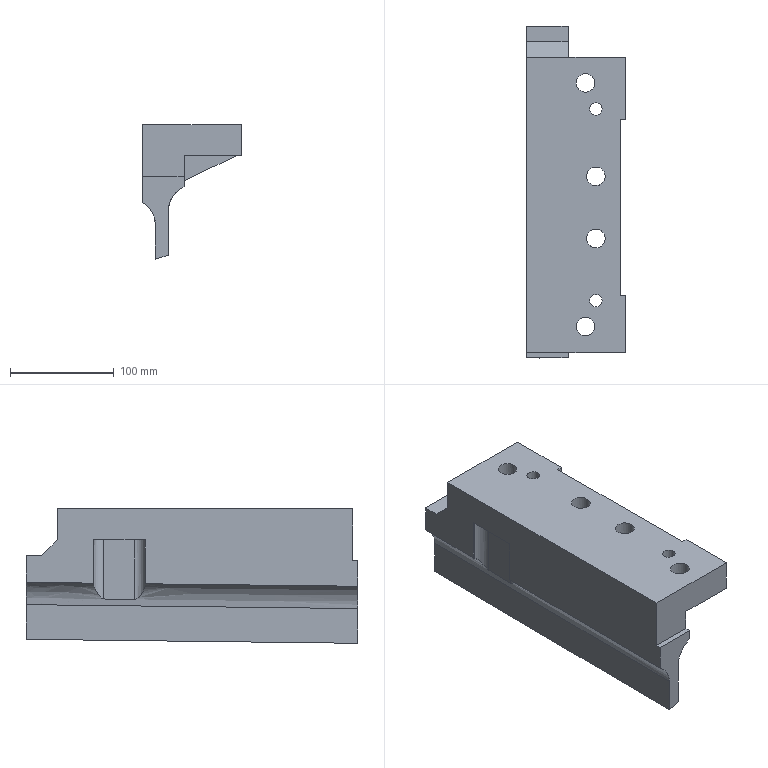Part | NX | features solid 2 | 1 solid | 55 faces | box 95.292 x 320 x 129.748 mm | volume 1453332 mm3 | plane 35 | cylinder 13 | spline 7 | commonest cylinder face diameters 18 x4 26 x4 12 x2 20 x2 10 x1